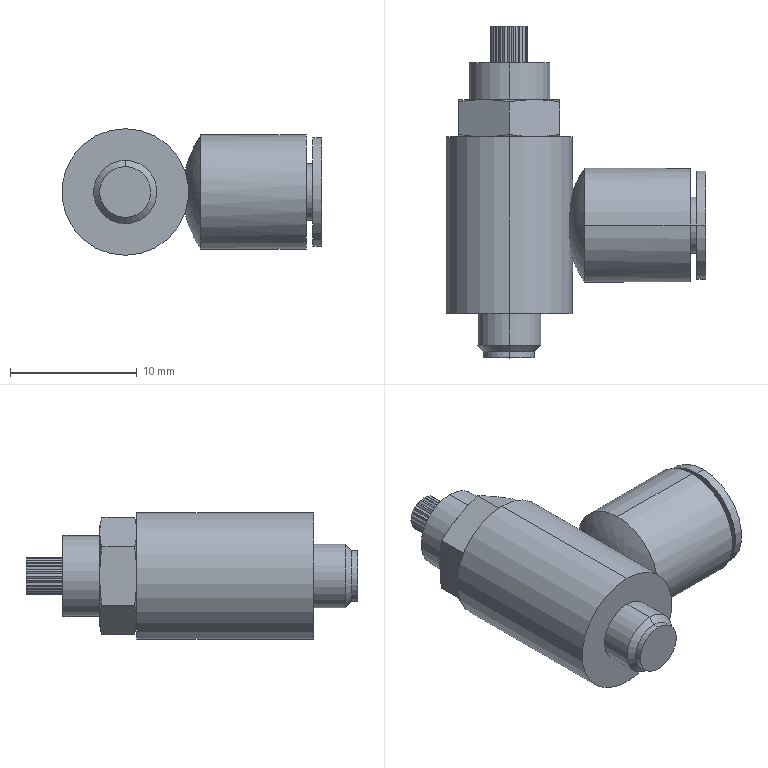Part | SolidWorks | features BaseBody 1 | 1 solid | 98 faces | box 20.5 x 26.2 x 10 mm | volume 1922 mm3 | plane 64 | cylinder 16 | cone 16 | spline 2 | commonest cylinder face diameters 4 x2 4.019 x2 4.444 x2 5 x2 6.4 x2 8.571 x2